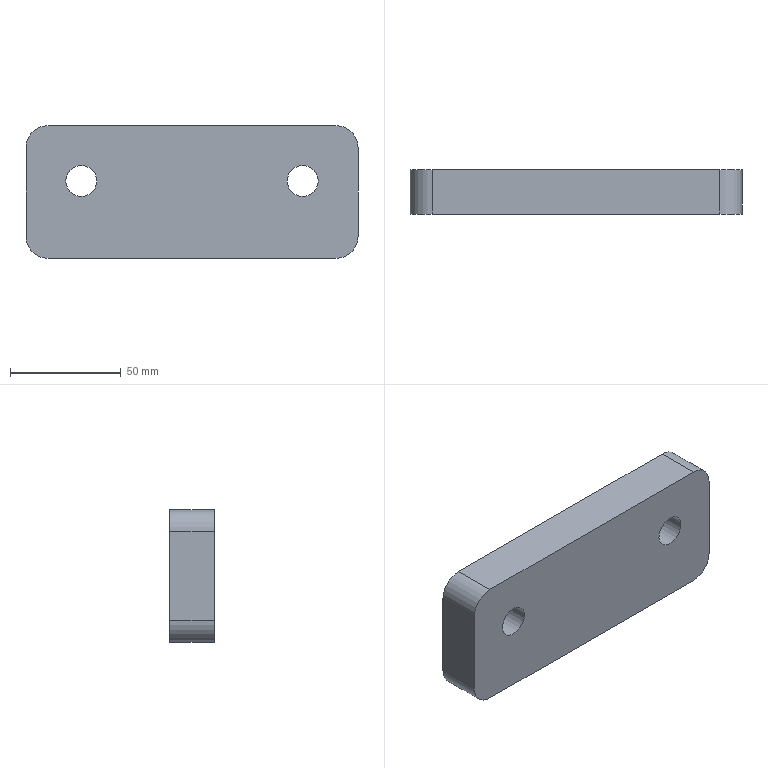Part | SolidWorks | features BaseBody 1 | 1 solid | 14 faces | box 150 x 20 x 60 mm | volume 172126 mm3 | cylinder 8 | plane 6 | commonest cylinder face diameters 14 x4 20 x4
STEP:
#1=CARTESIAN_POINT('',(-57.,-12.5,5.));
#2=VERTEX_POINT('',#1);
#3=CARTESIAN_POINT('',(-43.,-12.5,5.));
#4=VERTEX_POINT('',#3);
#5=CARTESIAN_POINT('',(-50.,-12.5,5.));
#6=DIRECTION('',(0.,-1.,0.));
#7=DIRECTION('',(0.,0.,-1.));
#8=AXIS2_PLACEMENT_3D('',#5,#6,#7);
#9=CIRCLE('',#8,7.);
#10=EDGE_CURVE('',#2,#4,#9,.T.);
#11=ORIENTED_EDGE('',*,*,#10,.T.);
#12=CARTESIAN_POINT('',(-43.,7.5,5.));
#13=VERTEX_POINT('',#12);
#14=CARTESIAN_POINT('',(-43.,7.5,5.));
#15=DIRECTION('',(0.,1.,0.));
#16=VECTOR('',#15,1000.);
#17=LINE('',#14,#16);
#18=EDGE_CURVE('',#4,#13,#17,.T.);
#19=ORIENTED_EDGE('',*,*,#18,.T.);
#20=CARTESIAN_POINT('',(-57.,7.5,5.));
#21=VERTEX_POINT('',#20);
#22=CARTESIAN_POINT('',(-50.,7.5,5.));
#23=DIRECTION('',(0.,1.,0.));
#24=DIRECTION('',(-1.,0.,0.));
#25=AXIS2_PLACEMENT_3D('',#22,#23,#24);
#26=CIRCLE('',#25,7.);
#27=EDGE_CURVE('',#13,#21,#26,.T.);
#28=ORIENTED_EDGE('',*,*,#27,.T.);
#29=CARTESIAN_POINT('',(-57.,7.5,5.));
#30=DIRECTION('',(0.,1.,0.));
#31=VECTOR('',#30,1000.);
#32=LINE('',#29,#31);
#33=EDGE_CURVE('',#2,#21,#32,.T.);
#34=ORIENTED_EDGE('',*,*,#33,.F.);
#35=EDGE_LOOP('',(#11,#19,#28,#34));
#36=FACE_OUTER_BOUND('',#35,.T.);
#37=CARTESIAN_POINT('',(-50.,7.5,5.));
#38=DIRECTION('',(0.,1.,0.));
#39=DIRECTION('',(-1.,0.,0.));
#40=AXIS2_PLACEMENT_3D('',#37,#38,#39);
#41=CYLINDRICAL_SURFACE('',#40,7.);
#42=ADVANCED_FACE('',(#36),#41,.F.);
#43=CARTESIAN_POINT('',(43.,-12.5,5.));
#44=VERTEX_POINT('',#43);
#45=CARTESIAN_POINT('',(57.,-12.5,5.));
#46=VERTEX_POINT('',#45);
#47=CARTESIAN_POINT('',(50.,-12.5,5.));
#48=DIRECTION('',(0.,-1.,0.));
#49=DIRECTION('',(0.,0.,-1.));
#50=AXIS2_PLACEMENT_3D('',#47,#48,#49);
#51=CIRCLE('',#50,7.);
#52=EDGE_CURVE('',#44,#46,#51,.T.);
#53=ORIENTED_EDGE('',*,*,#52,.T.);
#54=CARTESIAN_POINT('',(57.,7.5,5.));
#55=VERTEX_POINT('',#54);
#56=CARTESIAN_POINT('',(57.,7.5,5.));
#57=DIRECTION('',(0.,1.,0.));
#58=VECTOR('',#57,1000.);
#59=LINE('',#56,#58);
#60=EDGE_CURVE('',#46,#55,#59,.T.);
#61=ORIENTED_EDGE('',*,*,#60,.T.);
#62=CARTESIAN_POINT('',(43.,7.5,5.));
#63=VERTEX_POINT('',#62);
#64=CARTESIAN_POINT('',(50.,7.5,5.));
#65=DIRECTION('',(0.,1.,0.));
#66=DIRECTION('',(-1.,0.,0.));
#67=AXIS2_PLACEMENT_3D('',#64,#65,#66);
#68=CIRCLE('',#67,7.);
#69=EDGE_CURVE('',#55,#63,#68,.T.);
#70=ORIENTED_EDGE('',*,*,#69,.T.);
#71=CARTESIAN_POINT('',(43.,7.5,5.));
#72=DIRECTION('',(0.,1.,0.));
#73=VECTOR('',#72,1000.);
#74=LINE('',#71,#73);
#75=EDGE_CURVE('',#44,#63,#74,.T.);
#76=ORIENTED_EDGE('',*,*,#75,.F.);
#77=EDGE_LOOP('',(#53,#61,#70,#76));
#78=FACE_OUTER_BOUND('',#77,.T.);
#79=CARTESIAN_POINT('',(50.,7.5,5.));
#80=DIRECTION('',(0.,1.,0.));
#81=DIRECTION('',(-1.,0.,0.));
#82=AXIS2_PLACEMENT_3D('',#79,#80,#81);
#83=CYLINDRICAL_SURFACE('',#82,7.);
#84=ADVANCED_FACE('',(#78),#83,.F.);
#85=CARTESIAN_POINT('',(75.,7.5,-20.));
#86=VERTEX_POINT('',#85);
#87=CARTESIAN_POINT('',(65.,7.5,-30.));
#88=VERTEX_POINT('',#87);
#89=CARTESIAN_POINT('',(65.,7.5,-20.));
#90=DIRECTION('',(0.,1.,0.));
#91=DIRECTION('',(-1.,0.,0.));
#92=AXIS2_PLACEMENT_3D('',#89,#90,#91);
#93=CIRCLE('',#92,10.);
#94=EDGE_CURVE('',#86,#88,#93,.T.);
#95=ORIENTED_EDGE('',*,*,#94,.F.);
#96=CARTESIAN_POINT('',(75.,-12.5,-20.));
#97=VERTEX_POINT('',#96);
#98=CARTESIAN_POINT('',(75.,12.5,-20.));
#99=DIRECTION('',(0.,-1.,0.));
#100=VECTOR('',#99,1000.);
#101=LINE('',#98,#100);
#102=EDGE_CURVE('',#86,#97,#101,.T.);
#103=ORIENTED_EDGE('',*,*,#102,.T.);
#104=CARTESIAN_POINT('',(65.,-12.5,-30.));
#105=VERTEX_POINT('',#104);
#106=CARTESIAN_POINT('',(65.,-12.5,-20.));
#107=DIRECTION('',(0.,1.,0.));
#108=DIRECTION('',(0.,0.,-1.));
#109=AXIS2_PLACEMENT_3D('',#106,#107,#108);
#110=CIRCLE('',#109,10.);
#111=EDGE_CURVE('',#97,#105,#110,.T.);
#112=ORIENTED_EDGE('',*,*,#111,.T.);
#113=CARTESIAN_POINT('',(65.,12.5,-30.));
#114=DIRECTION('',(0.,-1.,0.));
#115=VECTOR('',#114,1000.);
#116=LINE('',#113,#115);
#117=EDGE_CURVE('',#88,#105,#116,.T.);
#118=ORIENTED_EDGE('',*,*,#117,.F.);
#119=EDGE_LOOP('',(#95,#103,#112,#118));
#120=FACE_OUTER_BOUND('',#119,.T.);
#121=CARTESIAN_POINT('',(65.,12.5,-20.));
#122=DIRECTION('',(0.,-1.,0.));
#123=DIRECTION('',(0.,0.,-1.));
#124=AXIS2_PLACEMENT_3D('',#121,#122,#123);
#125=CYLINDRICAL_SURFACE('',#124,10.);
#126=ADVANCED_FACE('',(#120),#125,.T.);
#127=CARTESIAN_POINT('',(-65.,7.5,-30.));
#128=VERTEX_POINT('',#127);
#129=CARTESIAN_POINT('',(65.,7.5,-30.));
#130=DIRECTION('',(-1.,0.,0.));
#131=VECTOR('',#130,1000.);
#132=LINE('',#129,#131);
#133=EDGE_CURVE('',#88,#128,#132,.T.);
#134=ORIENTED_EDGE('',*,*,#133,.F.);
#135=ORIENTED_EDGE('',*,*,#117,.T.);
#136=CARTESIAN_POINT('',(-65.,-12.5,-30.));
#137=VERTEX_POINT('',#136);
#138=CARTESIAN_POINT('',(-65.,-12.5,-30.));
#139=DIRECTION('',(-1.,0.,0.));
#140=VECTOR('',#139,1000.);
#141=LINE('',#138,#140);
#142=EDGE_CURVE('',#105,#137,#141,.T.);
#143=ORIENTED_EDGE('',*,*,#142,.T.);
#144=CARTESIAN_POINT('',(-65.,12.5,-30.));
#145=DIRECTION('',(0.,-1.,0.));
#146=VECTOR('',#145,1000.);
#147=LINE('',#144,#146);
#148=EDGE_CURVE('',#128,#137,#147,.T.);
#149=ORIENTED_EDGE('',*,*,#148,.F.);
#150=EDGE_LOOP('',(#134,#135,#143,#149));
#151=FACE_OUTER_BOUND('',#150,.T.);
#152=CARTESIAN_POINT('',(-65.,12.5,-30.));
#153=DIRECTION('',(0.,0.,1.));
#154=DIRECTION('',(1.,0.,0.));
#155=AXIS2_PLACEMENT_3D('',#152,#153,#154);
#156=PLANE('',#155);
#157=ADVANCED_FACE('',(#151),#156,.F.);
#158=CARTESIAN_POINT('',(-75.,7.5,-20.));
#159=VERTEX_POINT('',#158);
#160=CARTESIAN_POINT('',(-65.,7.5,-20.));
#161=DIRECTION('',(0.,1.,0.));
#162=DIRECTION('',(-1.,0.,0.));
#163=AXIS2_PLACEMENT_3D('',#160,#161,#162);
#164=CIRCLE('',#163,10.);
#165=EDGE_CURVE('',#128,#159,#164,.T.);
#166=ORIENTED_EDGE('',*,*,#165,.F.);
#167=ORIENTED_EDGE('',*,*,#148,.T.);
#168=CARTESIAN_POINT('',(-75.,-12.5,-20.));
#169=VERTEX_POINT('',#168);
#170=CARTESIAN_POINT('',(-65.,-12.5,-20.));
#171=DIRECTION('',(0.,1.,0.));
#172=DIRECTION('',(0.,0.,1.));
#173=AXIS2_PLACEMENT_3D('',#170,#171,#172);
#174=CIRCLE('',#173,10.);
#175=EDGE_CURVE('',#137,#169,#174,.T.);
#176=ORIENTED_EDGE('',*,*,#175,.T.);
#177=CARTESIAN_POINT('',(-75.,12.5,-20.));
#178=DIRECTION('',(0.,-1.,0.));
#179=VECTOR('',#178,1000.);
#180=LINE('',#177,#179);
#181=EDGE_CURVE('',#159,#169,#180,.T.);
#182=ORIENTED_EDGE('',*,*,#181,.F.);
#183=EDGE_LOOP('',(#166,#167,#176,#182));
#184=FACE_OUTER_BOUND('',#183,.T.);
#185=CARTESIAN_POINT('',(-65.,12.5,-20.));
#186=DIRECTION('',(0.,-1.,0.));
#187=DIRECTION('',(0.,0.,-1.));
#188=AXIS2_PLACEMENT_3D('',#185,#186,#187);
#189=CYLINDRICAL_SURFACE('',#188,10.);
#190=ADVANCED_FACE('',(#184),#189,.T.);
#191=CARTESIAN_POINT('',(-75.,7.5,20.));
#192=VERTEX_POINT('',#191);
#193=CARTESIAN_POINT('',(-75.,7.5,-20.));
#194=DIRECTION('',(0.,0.,1.));
#195=VECTOR('',#194,1000.);
#196=LINE('',#193,#195);
#197=EDGE_CURVE('',#159,#192,#196,.T.);
#198=ORIENTED_EDGE('',*,*,#197,.F.);
#199=ORIENTED_EDGE('',*,*,#181,.T.);
#200=CARTESIAN_POINT('',(-75.,-12.5,20.));
#201=VERTEX_POINT('',#200);
#202=CARTESIAN_POINT('',(-75.,-12.5,-20.));
#203=DIRECTION('',(0.,0.,1.));
#204=VECTOR('',#203,1000.);
#205=LINE('',#202,#204);
#206=EDGE_CURVE('',#169,#201,#205,.T.);
#207=ORIENTED_EDGE('',*,*,#206,.T.);
#208=CARTESIAN_POINT('',(-75.,12.5,20.));
#209=DIRECTION('',(0.,-1.,0.));
#210=VECTOR('',#209,1000.);
#211=LINE('',#208,#210);
#212=EDGE_CURVE('',#192,#201,#211,.T.);
#213=ORIENTED_EDGE('',*,*,#212,.F.);
#214=EDGE_LOOP('',(#198,#199,#207,#213));
#215=FACE_OUTER_BOUND('',#214,.T.);
#216=CARTESIAN_POINT('',(-75.,12.5,-20.));
#217=DIRECTION('',(1.,0.,0.));
#218=DIRECTION('',(0.,0.,-1.));
#219=AXIS2_PLACEMENT_3D('',#216,#217,#218);
#220=PLANE('',#219);
#221=ADVANCED_FACE('',(#215),#220,.F.);
#222=CARTESIAN_POINT('',(-65.,7.5,30.));
#223=VERTEX_POINT('',#222);
#224=CARTESIAN_POINT('',(-65.,7.5,20.));
#225=DIRECTION('',(0.,1.,0.));
#226=DIRECTION('',(-1.,0.,0.));
#227=AXIS2_PLACEMENT_3D('',#224,#225,#226);
#228=CIRCLE('',#227,10.);
#229=EDGE_CURVE('',#192,#223,#228,.T.);
#230=ORIENTED_EDGE('',*,*,#229,.F.);
#231=ORIENTED_EDGE('',*,*,#212,.T.);
#232=CARTESIAN_POINT('',(-65.,-12.5,30.));
#233=VERTEX_POINT('',#232);
#234=CARTESIAN_POINT('',(-65.,-12.5,20.));
#235=DIRECTION('',(0.,1.,0.));
#236=DIRECTION('',(0.,0.,1.));
#237=AXIS2_PLACEMENT_3D('',#234,#235,#236);
#238=CIRCLE('',#237,10.);
#239=EDGE_CURVE('',#201,#233,#238,.T.);
#240=ORIENTED_EDGE('',*,*,#239,.T.);
#241=CARTESIAN_POINT('',(-65.,12.5,30.));
#242=DIRECTION('',(0.,-1.,0.));
#243=VECTOR('',#242,1000.);
#244=LINE('',#241,#243);
#245=EDGE_CURVE('',#223,#233,#244,.T.);
#246=ORIENTED_EDGE('',*,*,#245,.F.);
#247=EDGE_LOOP('',(#230,#231,#240,#246));
#248=FACE_OUTER_BOUND('',#247,.T.);
#249=CARTESIAN_POINT('',(-65.,12.5,20.));
#250=DIRECTION('',(0.,-1.,0.));
#251=DIRECTION('',(0.,0.,-1.));
#252=AXIS2_PLACEMENT_3D('',#249,#250,#251);
#253=CYLINDRICAL_SURFACE('',#252,10.);
#254=ADVANCED_FACE('',(#248),#253,.T.);
#255=CARTESIAN_POINT('',(65.,7.5,30.));
#256=VERTEX_POINT('',#255);
#257=CARTESIAN_POINT('',(-65.,7.5,30.));
#258=DIRECTION('',(1.,0.,0.));
#259=VECTOR('',#258,1000.);
#260=LINE('',#257,#259);
#261=EDGE_CURVE('',#223,#256,#260,.T.);
#262=ORIENTED_EDGE('',*,*,#261,.F.);
#263=ORIENTED_EDGE('',*,*,#245,.T.);
#264=CARTESIAN_POINT('',(65.,-12.5,30.));
#265=VERTEX_POINT('',#264);
#266=CARTESIAN_POINT('',(-65.,-12.5,30.));
#267=DIRECTION('',(1.,0.,0.));
#268=VECTOR('',#267,1000.);
#269=LINE('',#266,#268);
#270=EDGE_CURVE('',#233,#265,#269,.T.);
#271=ORIENTED_EDGE('',*,*,#270,.T.);
#272=CARTESIAN_POINT('',(65.,12.5,30.));
#273=DIRECTION('',(0.,-1.,0.));
#274=VECTOR('',#273,1000.);
#275=LINE('',#272,#274);
#276=EDGE_CURVE('',#256,#265,#275,.T.);
#277=ORIENTED_EDGE('',*,*,#276,.F.);
#278=EDGE_LOOP('',(#262,#263,#271,#277));
#279=FACE_OUTER_BOUND('',#278,.T.);
#280=CARTESIAN_POINT('',(-65.,12.5,30.));
#281=DIRECTION('',(0.,0.,-1.));
#282=DIRECTION('',(-1.,0.,0.));
#283=AXIS2_PLACEMENT_3D('',#280,#281,#282);
#284=PLANE('',#283);
#285=ADVANCED_FACE('',(#279),#284,.F.);
#286=CARTESIAN_POINT('',(75.,7.5,20.));
#287=VERTEX_POINT('',#286);
#288=CARTESIAN_POINT('',(65.,7.5,20.));
#289=DIRECTION('',(0.,1.,0.));
#290=DIRECTION('',(-1.,0.,0.));
#291=AXIS2_PLACEMENT_3D('',#288,#289,#290);
#292=CIRCLE('',#291,10.);
#293=EDGE_CURVE('',#256,#287,#292,.T.);
#294=ORIENTED_EDGE('',*,*,#293,.F.);
#295=ORIENTED_EDGE('',*,*,#276,.T.);
#296=CARTESIAN_POINT('',(75.,-12.5,20.));
#297=VERTEX_POINT('',#296);
#298=CARTESIAN_POINT('',(65.,-12.5,20.));
#299=DIRECTION('',(0.,1.,0.));
#300=DIRECTION('',(0.,0.,1.));
#301=AXIS2_PLACEMENT_3D('',#298,#299,#300);
#302=CIRCLE('',#301,10.);
#303=EDGE_CURVE('',#265,#297,#302,.T.);
#304=ORIENTED_EDGE('',*,*,#303,.T.);
#305=CARTESIAN_POINT('',(75.,12.5,20.));
#306=DIRECTION('',(0.,-1.,0.));
#307=VECTOR('',#306,1000.);
#308=LINE('',#305,#307);
#309=EDGE_CURVE('',#287,#297,#308,.T.);
#310=ORIENTED_EDGE('',*,*,#309,.F.);
#311=EDGE_LOOP('',(#294,#295,#304,#310));
#312=FACE_OUTER_BOUND('',#311,.T.);
#313=CARTESIAN_POINT('',(65.,12.5,20.));
#314=DIRECTION('',(0.,-1.,0.));
#315=DIRECTION('',(0.,0.,-1.));
#316=AXIS2_PLACEMENT_3D('',#313,#314,#315);
#317=CYLINDRICAL_SURFACE('',#316,10.);
#318=ADVANCED_FACE('',(#312),#317,.T.);
#319=CARTESIAN_POINT('',(75.,7.5,20.));
#320=DIRECTION('',(0.,0.,-1.));
#321=VECTOR('',#320,1000.);
#322=LINE('',#319,#321);
#323=EDGE_CURVE('',#287,#86,#322,.T.);
#324=ORIENTED_EDGE('',*,*,#323,.F.);
#325=ORIENTED_EDGE('',*,*,#309,.T.);
#326=CARTESIAN_POINT('',(75.,-12.5,-20.));
#327=DIRECTION('',(0.,0.,-1.));
#328=VECTOR('',#327,1000.);
#329=LINE('',#326,#328);
#330=EDGE_CURVE('',#297,#97,#329,.T.);
#331=ORIENTED_EDGE('',*,*,#330,.T.);
#332=ORIENTED_EDGE('',*,*,#102,.F.);
#333=EDGE_LOOP('',(#324,#325,#331,#332));
#334=FACE_OUTER_BOUND('',#333,.T.);
#335=CARTESIAN_POINT('',(75.,12.5,-20.));
#336=DIRECTION('',(-1.,0.,0.));
#337=DIRECTION('',(0.,0.,1.));
#338=AXIS2_PLACEMENT_3D('',#335,#336,#337);
#339=PLANE('',#338);
#340=ADVANCED_FACE('',(#334),#339,.F.);
#341=ORIENTED_EDGE('',*,*,#10,.F.);
#342=CARTESIAN_POINT('',(-50.,-12.5,5.));
#343=DIRECTION('',(0.,-1.,0.));
#344=DIRECTION('',(0.,0.,-1.));
#345=AXIS2_PLACEMENT_3D('',#342,#343,#344);
#346=CIRCLE('',#345,7.);
#347=EDGE_CURVE('',#4,#2,#346,.T.);
#348=ORIENTED_EDGE('',*,*,#347,.F.);
#349=EDGE_LOOP('',(#341,#348));
#350=FACE_BOUND('',#349,.T.);
#351=ORIENTED_EDGE('',*,*,#52,.F.);
#352=CARTESIAN_POINT('',(50.,-12.5,5.));
#353=DIRECTION('',(0.,-1.,0.));
#354=DIRECTION('',(0.,0.,-1.));
#355=AXIS2_PLACEMENT_3D('',#352,#353,#354);
#356=CIRCLE('',#355,7.);
#357=EDGE_CURVE('',#46,#44,#356,.T.);
#358=ORIENTED_EDGE('',*,*,#357,.F.);
#359=EDGE_LOOP('',(#351,#358));
#360=FACE_BOUND('',#359,.T.);
#361=ORIENTED_EDGE('',*,*,#111,.F.);
#362=ORIENTED_EDGE('',*,*,#330,.F.);
#363=ORIENTED_EDGE('',*,*,#303,.F.);
#364=ORIENTED_EDGE('',*,*,#270,.F.);
#365=ORIENTED_EDGE('',*,*,#239,.F.);
#366=ORIENTED_EDGE('',*,*,#206,.F.);
#367=ORIENTED_EDGE('',*,*,#175,.F.);
#368=ORIENTED_EDGE('',*,*,#142,.F.);
#369=EDGE_LOOP('',(#361,#362,#363,#364,#365,#366,#367,#368));
#370=FACE_OUTER_BOUND('',#369,.T.);
#371=CARTESIAN_POINT('',(65.,-12.5,-20.));
#372=DIRECTION('',(0.,-1.,0.));
#373=DIRECTION('',(0.,0.,-1.));
#374=AXIS2_PLACEMENT_3D('',#371,#372,#373);
#375=PLANE('',#374);
#376=ADVANCED_FACE('',(#350,#360,#370),#375,.T.);
#377=CARTESIAN_POINT('',(-50.,7.5,5.));
#378=DIRECTION('',(0.,1.,0.));
#379=DIRECTION('',(-1.,0.,0.));
#380=AXIS2_PLACEMENT_3D('',#377,#378,#379);
#381=CIRCLE('',#380,7.);
#382=EDGE_CURVE('',#21,#13,#381,.T.);
#383=ORIENTED_EDGE('',*,*,#382,.F.);
#384=ORIENTED_EDGE('',*,*,#27,.F.);
#385=EDGE_LOOP('',(#383,#384));
#386=FACE_BOUND('',#385,.T.);
#387=CARTESIAN_POINT('',(50.,7.5,5.));
#388=DIRECTION('',(0.,1.,0.));
#389=DIRECTION('',(-1.,0.,0.));
#390=AXIS2_PLACEMENT_3D('',#387,#388,#389);
#391=CIRCLE('',#390,7.);
#392=EDGE_CURVE('',#63,#55,#391,.T.);
#393=ORIENTED_EDGE('',*,*,#392,.F.);
#394=ORIENTED_EDGE('',*,*,#69,.F.);
#395=EDGE_LOOP('',(#393,#394));
#396=FACE_BOUND('',#395,.T.);
#397=ORIENTED_EDGE('',*,*,#94,.T.);
#398=ORIENTED_EDGE('',*,*,#133,.T.);
#399=ORIENTED_EDGE('',*,*,#165,.T.);
#400=ORIENTED_EDGE('',*,*,#197,.T.);
#401=ORIENTED_EDGE('',*,*,#229,.T.);
#402=ORIENTED_EDGE('',*,*,#261,.T.);
#403=ORIENTED_EDGE('',*,*,#293,.T.);
#404=ORIENTED_EDGE('',*,*,#323,.T.);
#405=EDGE_LOOP('',(#397,#398,#399,#400,#401,#402,#403,#404));
#406=FACE_OUTER_BOUND('',#405,.T.);
#407=CARTESIAN_POINT('',(65.,7.5,-20.));
#408=DIRECTION('',(0.,1.,0.));
#409=DIRECTION('',(-1.,0.,0.));
#410=AXIS2_PLACEMENT_3D('',#407,#408,#409);
#411=PLANE('',#410);
#412=ADVANCED_FACE('',(#386,#396,#406),#411,.T.);
#413=ORIENTED_EDGE('',*,*,#60,.F.);
#414=ORIENTED_EDGE('',*,*,#357,.T.);
#415=ORIENTED_EDGE('',*,*,#75,.T.);
#416=ORIENTED_EDGE('',*,*,#392,.T.);
#417=EDGE_LOOP('',(#413,#414,#415,#416));
#418=FACE_OUTER_BOUND('',#417,.T.);
#419=CARTESIAN_POINT('',(50.,7.5,5.));
#420=DIRECTION('',(0.,1.,0.));
#421=DIRECTION('',(-1.,0.,0.));
#422=AXIS2_PLACEMENT_3D('',#419,#420,#421);
#423=CYLINDRICAL_SURFACE('',#422,7.);
#424=ADVANCED_FACE('',(#418),#423,.F.);
#425=ORIENTED_EDGE('',*,*,#18,.F.);
#426=ORIENTED_EDGE('',*,*,#347,.T.);
#427=ORIENTED_EDGE('',*,*,#33,.T.);
#428=ORIENTED_EDGE('',*,*,#382,.T.);
#429=EDGE_LOOP('',(#425,#426,#427,#428));
#430=FACE_OUTER_BOUND('',#429,.T.);
#431=CARTESIAN_POINT('',(-50.,7.5,5.));
#432=DIRECTION('',(0.,1.,0.));
#433=DIRECTION('',(-1.,0.,0.));
#434=AXIS2_PLACEMENT_3D('',#431,#432,#433);
#435=CYLINDRICAL_SURFACE('',#434,7.);
#436=ADVANCED_FACE('',(#430),#435,.F.);
#437=CLOSED_SHELL('',(#42,#84,#126,#157,#190,#221,#254,#285,#318,#340,#376,#412,#424,#436));
#438=MANIFOLD_SOLID_BREP('',#437);
#439=CARTESIAN_POINT('',(0.,0.,0.));
#440=DIRECTION('',(0.,0.,1.));
#441=DIRECTION('',(1.,0.,0.));
#442=AXIS2_PLACEMENT_3D('',#439,#440,#441);
#443=(LENGTH_UNIT()NAMED_UNIT(*)SI_UNIT(.MILLI.,.METRE.));
#444=UNCERTAINTY_MEASURE_WITH_UNIT(LENGTH_MEASURE(0.00001),#443,'','');
#445=(NAMED_UNIT(*)PLANE_ANGLE_UNIT()SI_UNIT($,.RADIAN.));
#446=(NAMED_UNIT(*)SI_UNIT($,.STERADIAN.)SOLID_ANGLE_UNIT());
#447=(GEOMETRIC_REPRESENTATION_CONTEXT(3)GLOBAL_UNCERTAINTY_ASSIGNED_CONTEXT((#444))GLOBAL_UNIT_ASSIGNED_CONTEXT((#443,#445,#446))REPRESENTATION_CONTEXT('',''));
#448=ADVANCED_BREP_SHAPE_REPRESENTATION('',(#438,#442),#447);